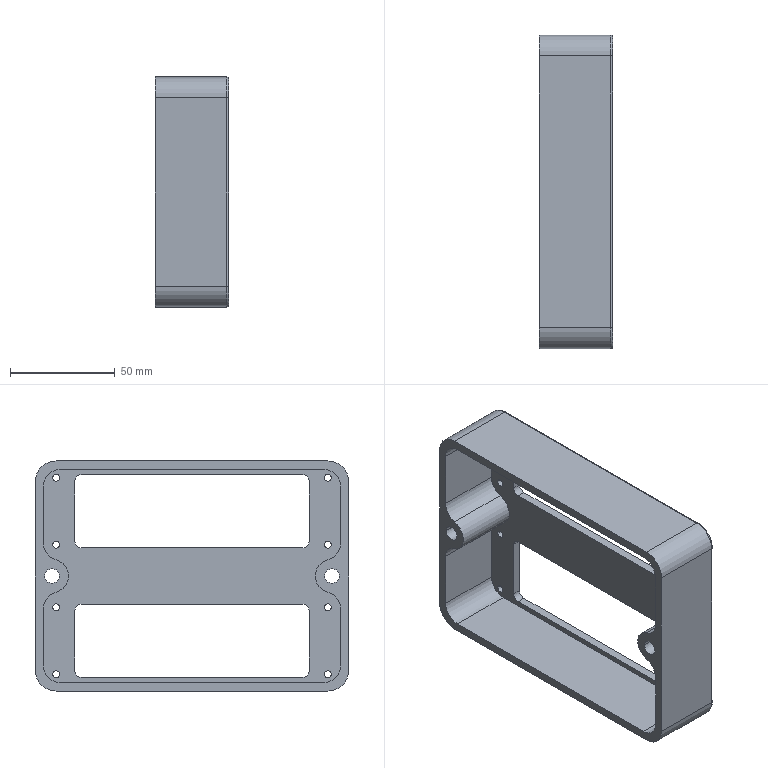Part | STEP file | CN-WB(CN-WB24x24) | 1 solid | 78 faces | box 35 x 150 x 110 mm | volume 103004 mm3 | cylinder 51 | plane 23 | torus 4 | commonest cylinder face diameters 3.3 x16 16 x11 6 x8 2 x4 7 x4 12 x4